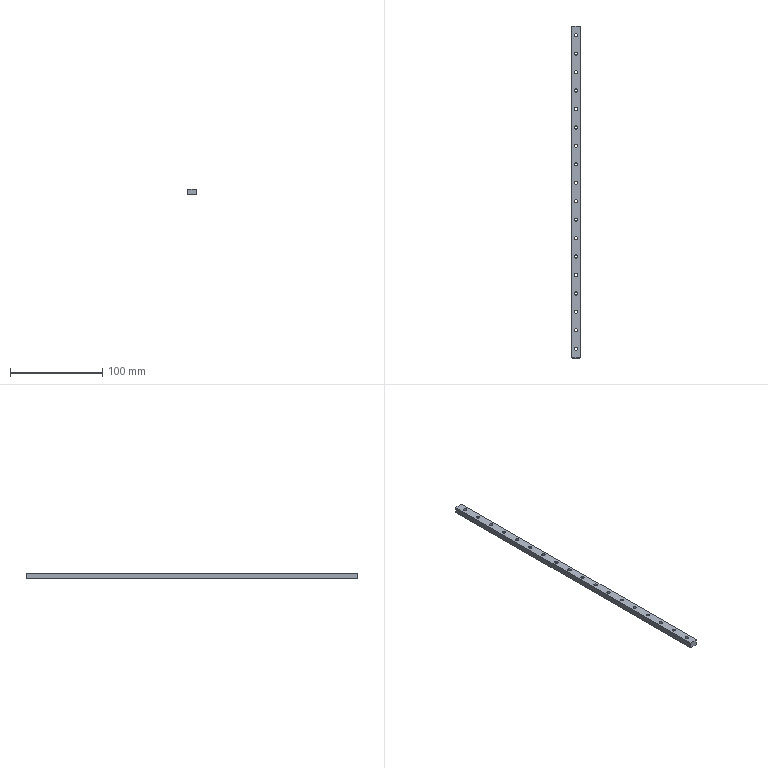Part | SolidWorks | features ICE 2, LPattern 2, Chamfer 1, Extrusion 1 | 1 solid | 98 faces | box 9 x 360 x 6.5 mm | volume 18391 mm3 | cylinder 72 | plane 26 | commonest cylinder face diameters 3.5 x36 6 x36